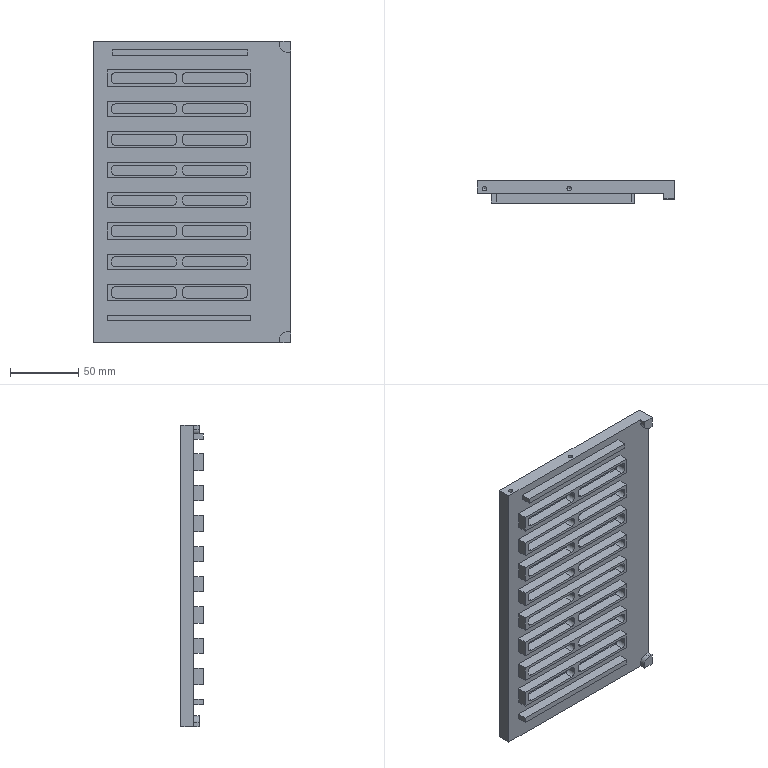NC program | NX | posted with a generic post | part box 144.5 x 16.5 x 221 mm
Whole program:
N10 G17 G21 G94 G90
(DRILLING , TOOL : D8-120)
N12 T19 M6
N14 G54
N16 G17 G0 G90 X-100.5 Y-6. B0. C0. S2000 M3
N18 G43 Z20. H19
N20 G94 G81 G99 Z-0.9 B-180. C-90. F200. R3.
N22 X-32.5
N24 X32.5
N26 X100.5
N28 G80
N30 G0 X100.5 Y-6. Z20.
N32 M5
(DRILLING_COPY , TOOL : 钻头D3.3-45-73)
N34 T09 M6
N36 G54
N38 G17 G0 G90 X-100.5 Y-6. B0. C0. S2000 M3
N40 G43 Z20. H9
N42 G94 G81 G99 Z-9.45 B-180. C-90. F200. R3.
N44 X-32.5
N46 X32.5
N48 X100.5
N50 G80
N52 G0 X100.5 Y-6. Z20.
N54 M5
(DRILLING_COPY_COPY , TOOL : D3.3插刀)
N56 T10 M6
N58 G54
N60 G17 G0 G90 X-100.5 Y-6. B0. C0. S2000 M3
N62 G43 Z20. H10
N64 G94 G81 G99 Z-9.5 B-180. C-90. F200. R3.
N66 X-32.5
N68 X32.5
N70 X100.5
N72 G80
N74 G0 X100.5 Y-6. Z20.
N76 M5
(THREAD_MILLING , TOOL : THREAD_MILL)
N78 T11 M6
N80 G54
N82 G17 G0 G90 X-100.5 Y-6. B0. C0. S3000 M3
N84 G43 Z20. H11
N86 Z-8.675 B-180. C-90.
N88 G41 G94 G3 X-100.35 Y-5.88 Z-8.5 I0.075 J0.06 F200. D11
N90 X-100.35 Y-5.88 Z-7.8 I-0.15 J-0.12
N92 X-100.5 Y-6. Z-7.625 I-0.075 J-0.06
N94 G40
N96 G0 Z-7.275
N98 G41 G3 X-100.35 Y-5.88 Z-7.1 I0.075 J0.06
N100 X-100.35 Y-5.88 Z-6.4 I-0.15 J-0.12
N102 X-100.5 Y-6. Z-6.225 I-0.075 J-0.06
N104 G40
N106 G0 Z-5.875
N108 G41 G3 X-100.35 Y-5.88 Z-5.7 I0.075 J0.06
N110 X-100.35 Y-5.88 Z-5. I-0.15 J-0.12
N112 X-100.5 Y-6. Z-4.825 I-0.075 J-0.06
N114 G40
N116 G0 Z-4.475
N118 G41 G3 X-100.35 Y-5.88 Z-4.3 I0.075 J0.06
N120 X-100.35 Y-5.88 Z-3.6 I-0.15 J-0.12
N122 X-100.5 Y-6. Z-3.425 I-0.075 J-0.06
N124 G40
N126 G0 Z-3.075
N128 G41 G3 X-100.35 Y-5.88 Z-2.9 I0.075 J0.06
N130 X-100.35 Y-5.88 Z-2.2 I-0.15 J-0.12
N132 X-100.5 Y-6. Z-2.025 I-0.075 J-0.06
N134 G40
N136 G0 Z-1.675
N138 G41 G3 X-100.35 Y-5.88 Z-1.5 I0.075 J0.06
N140 X-100.35 Y-5.88 Z-0.8 I-0.15 J-0.12
N142 X-100.35 Y-5.88 Z-0.1 I-0.15 J-0.12
N144 X-100.583 Y-6.173 Z0.3 R-0.192
N146 X-100.5 Y-6. Z0.475 I0.042 J0.086
N148 G40
N150 G0 Z-8.675
N152 G41 G3 X-100.259 Y-5.808 Z-8.5 I0.121 J0.096
N154 X-100.259 Y-5.808 Z-7.8 I-0.241 J-0.192
N156 X-100.5 Y-6. Z-7.625 I-0.121 J-0.096
N158 G40
N160 G0 Z-7.275
N162 G41 G3 X-100.259 Y-5.808 Z-7.1 I0.121 J0.096
N164 X-100.259 Y-5.808 Z-6.4 I-0.241 J-0.192
N166 X-100.5 Y-6. Z-6.225 I-0.121 J-0.096
N168 G40
N170 G0 Z-5.875
N172 G41 G3 X-100.259 Y-5.808 Z-5.7 I0.121 J0.096
N174 X-100.259 Y-5.808 Z-5. I-0.241 J-0.192
N176 X-100.5 Y-6. Z-4.825 I-0.121 J-0.096
N178 G40
N180 G0 Z-4.475
N182 G41 G3 X-100.259 Y-5.808 Z-4.3 I0.121 J0.096
N184 X-100.259 Y-5.808 Z-3.6 I-0.241 J-0.192
N186 X-100.5 Y-6. Z-3.425 I-0.121 J-0.096
N188 G40
N190 G0 Z-3.075
N192 G41 G3 X-100.259 Y-5.808 Z-2.9 I0.121 J0.096
N194 X-100.259 Y-5.808 Z-2.2 I-0.241 J-0.192
N196 X-100.5 Y-6. Z-2.025 I-0.121 J-0.096
N198 G40
N200 G0 Z-1.675
N202 G41 G3 X-100.259 Y-5.808 Z-1.5 I0.121 J0.096
N204 X-100.259 Y-5.808 Z-0.8 I-0.241 J-0.192
N206 X-100.259 Y-5.808 Z-0.1 I-0.241 J-0.192
N208 X-100.634 Y-6.278 Z0.3 R-0.308
N210 X-100.5 Y-6. Z0.475 I0.067 J0.139
N212 G40
N214 G0 Z-8.557
N216 G41 G1 X-100.211 Y-5.921
N218 G3 X-100.168 Y-5.735 Z-8.5 R0.122
N220 X-100.168 Y-5.735 Z-7.8 I-0.332 J-0.265
N222 X-100.358 Y-5.736 Z-7.743 R0.122
N224 G40
N226 G1 X-100.5 Y-6.
N228 G0 Z-7.157
N230 G41 G1 X-100.211 Y-5.921
N232 G3 X-100.168 Y-5.735 Z-7.1 R0.122
N234 X-100.168 Y-5.735 Z-6.4 I-0.332 J-0.265
N236 X-100.358 Y-5.736 Z-6.343 R0.122
N238 G40
N240 G1 X-100.5 Y-6.
N242 G0 Z-5.757
N244 G41 G1 X-100.211 Y-5.921
N246 G3 X-100.168 Y-5.735 Z-5.7 R0.122
N248 X-100.168 Y-5.735 Z-5. I-0.332 J-0.265
N250 X-100.358 Y-5.736 Z-4.943 R0.122
N252 G40
N254 G1 X-100.5 Y-6.
N256 G0 Z-4.357
N258 G41 G1 X-100.211 Y-5.921
N260 G3 X-100.168 Y-5.735 Z-4.3 R0.122
N262 X-100.168 Y-5.735 Z-3.6 I-0.332 J-0.265
N264 X-100.358 Y-5.736 Z-3.543 R0.122
N266 G40
N268 G1 X-100.5 Y-6.
N270 G0 Z-2.957
N272 G41 G1 X-100.211 Y-5.921
N274 G3 X-100.168 Y-5.735 Z-2.9 R0.122
N276 X-100.168 Y-5.735 Z-2.2 I-0.332 J-0.265
N278 X-100.358 Y-5.736 Z-2.143 R0.122
N280 G40
N282 G1 X-100.5 Y-6.
N284 G0 Z-1.557
N286 G41 G1 X-100.211 Y-5.921
N288 G3 X-100.168 Y-5.735 Z-1.5 R0.122
N290 X-100.168 Y-5.735 Z-0.8 I-0.332 J-0.265
N292 X-100.168 Y-5.735 Z-0.1 I-0.332 J-0.265
N294 X-100.684 Y-6.383 Z0.3 R-0.425
N296 X-100.513 Y-6.3 Z0.357 R0.122
N298 G40
N300 G1 X-100.5 Y-6.
N302 G0 Z20.
N304 X-32.5
N306 Z-8.675
N308 G41 G3 X-32.35 Y-5.88 Z-8.5 I0.075 J0.06
N310 X-32.35 Y-5.88 Z-7.8 I-0.15 J-0.12
N312 X-32.5 Y-6. Z-7.625 I-0.075 J-0.06
N314 G40
N316 G0 Z-7.275
N318 G41 G3 X-32.35 Y-5.88 Z-7.1 I0.075 J0.06
N320 X-32.35 Y-5.88 Z-6.4 I-0.15 J-0.12
N322 X-32.5 Y-6. Z-6.225 I-0.075 J-0.06
N324 G40
N326 G0 Z-5.875
N328 G41 G3 X-32.35 Y-5.88 Z-5.7 I0.075 J0.06
N330 X-32.35 Y-5.88 Z-5. I-0.15 J-0.12
N332 X-32.5 Y-6. Z-4.825 I-0.075 J-0.06
N334 G40
N336 G0 Z-4.475
N338 G41 G3 X-32.35 Y-5.88 Z-4.3 I0.075 J0.06
N340 X-32.35 Y-5.88 Z-3.6 I-0.15 J-0.12
N342 X-32.5 Y-6. Z-3.425 I-0.075 J-0.06
N344 G40
N346 G0 Z-3.075
N348 G41 G3 X-32.35 Y-5.88 Z-2.9 I0.075 J0.06
N350 X-32.35 Y-5.88 Z-2.2 I-0.15 J-0.12
N352 X-32.5 Y-6. Z-2.025 I-0.075 J-0.06
N354 G40
N356 G0 Z-1.675
N358 G41 G3 X-32.35 Y-5.88 Z-1.5 I0.075 J0.06
N360 X-32.35 Y-5.88 Z-0.8 I-0.15 J-0.12
N362 X-32.35 Y-5.88 Z-0.1 I-0.15 J-0.12
N364 X-32.583 Y-6.173 Z0.3 R-0.192
N366 X-32.5 Y-6. Z0.475 I0.042 J0.086
N368 G40
N370 G0 Z-8.675
N372 G41 G3 X-32.259 Y-5.808 Z-8.5 I0.121 J0.096
N374 X-32.259 Y-5.808 Z-7.8 I-0.241 J-0.192
N376 X-32.5 Y-6. Z-7.625 I-0.121 J-0.096
N378 G40
N380 G0 Z-7.275
N382 G41 G3 X-32.259 Y-5.808 Z-7.1 I0.121 J0.096
N384 X-32.259 Y-5.808 Z-6.4 I-0.241 J-0.192
N386 X-32.5 Y-6. Z-6.225 I-0.121 J-0.096
N388 G40
N390 G0 Z-5.875
N392 G41 G3 X-32.259 Y-5.808 Z-5.7 I0.121 J0.096
N394 X-32.259 Y-5.808 Z-5. I-0.241 J-0.192
N396 X-32.5 Y-6. Z-4.825 I-0.121 J-0.096
N398 G40
N400 G0 Z-4.475
N402 G41 G3 X-32.259 Y-5.808 Z-4.3 I0.121 J0.096
N404 X-32.259 Y-5.808 Z-3.6 I-0.241 J-0.192
N406 X-32.5 Y-6. Z-3.425 I-0.121 J-0.096
N408 G40
N410 G0 Z-3.075
N412 G41 G3 X-32.259 Y-5.808 Z-2.9 I0.121 J0.096
N414 X-32.259 Y-5.808 Z-2.2 I-0.241 J-0.192
N416 X-32.5 Y-6. Z-2.025 I-0.121 J-0.096
N418 G40
N420 G0 Z-1.675
N422 G41 G3 X-32.259 Y-5.808 Z-1.5 I0.121 J0.096
N424 X-32.259 Y-5.808 Z-0.8 I-0.241 J-0.192
N426 X-32.259 Y-5.808 Z-0.1 I-0.241 J-0.192
N428 X-32.634 Y-6.278 Z0.3 R-0.308
N430 X-32.5 Y-6. Z0.475 I0.067 J0.139
N432 G40
N434 G0 Z-8.557
N436 G41 G1 X-32.211 Y-5.921
N438 G3 X-32.168 Y-5.735 Z-8.5 R0.122
N440 X-32.168 Y-5.735 Z-7.8 I-0.332 J-0.265
N442 X-32.358 Y-5.736 Z-7.743 R0.122
N444 G40
N446 G1 X-32.5 Y-6.
N448 G0 Z-7.157
N450 G41 G1 X-32.211 Y-5.921
N452 G3 X-32.168 Y-5.735 Z-7.1 R0.122
N454 X-32.168 Y-5.735 Z-6.4 I-0.332 J-0.265
N456 X-32.358 Y-5.736 Z-6.343 R0.122
N458 G40
N460 G1 X-32.5 Y-6.
N462 G0 Z-5.757
N464 G41 G1 X-32.211 Y-5.921
N466 G3 X-32.168 Y-5.735 Z-5.7 R0.122
N468 X-32.168 Y-5.735 Z-5. I-0.332 J-0.265
N470 X-32.358 Y-5.736 Z-4.943 R0.122
N472 G40
N474 G1 X-32.5 Y-6.
N476 G0 Z-4.357
N478 G41 G1 X-32.211 Y-5.921
N480 G3 X-32.168 Y-5.735 Z-4.3 R0.122
N482 X-32.168 Y-5.735 Z-3.6 I-0.332 J-0.265
N484 X-32.358 Y-5.736 Z-3.543 R0.122
N486 G40
N488 G1 X-32.5 Y-6.
N490 G0 Z-2.957
N492 G41 G1 X-32.211 Y-5.921
N494 G3 X-32.168 Y-5.735 Z-2.9 R0.122
N496 X-32.168 Y-5.735 Z-2.2 I-0.332 J-0.265
N498 X-32.358 Y-5.736 Z-2.143 R0.122
N500 G40
N502 G1 X-32.5 Y-6.
N504 G0 Z-1.557
N506 G41 G1 X-32.211 Y-5.921
N508 G3 X-32.168 Y-5.735 Z-1.5 R0.122
N510 X-32.168 Y-5.735 Z-0.8 I-0.332 J-0.265
N512 X-32.168 Y-5.735 Z-0.1 I-0.332 J-0.265
N514 X-32.684 Y-6.383 Z0.3 R-0.425
N516 X-32.513 Y-6.3 Z0.357 R0.122
N518 G40
N520 G1 X-32.5 Y-6.
N522 G0 Z20.
N524 X32.5
N526 Z-8.675
N528 G41 G3 X32.65 Y-5.88 Z-8.5 I0.075 J0.06
N530 X32.65 Y-5.88 Z-7.8 I-0.15 J-0.12
N532 X32.5 Y-6. Z-7.625 I-0.075 J-0.06
N534 G40
N536 G0 Z-7.275
N538 G41 G3 X32.65 Y-5.88 Z-7.1 I0.075 J0.06
N540 X32.65 Y-5.88 Z-6.4 I-0.15 J-0.12
N542 X32.5 Y-6. Z-6.225 I-0.075 J-0.06
N544 G40
N546 G0 Z-5.875
N548 G41 G3 X32.65 Y-5.88 Z-5.7 I0.075 J0.06
N550 X32.65 Y-5.88 Z-5. I-0.15 J-0.12
N552 X32.5 Y-6. Z-4.825 I-0.075 J-0.06
N554 G40
N556 G0 Z-4.475
N558 G41 G3 X32.65 Y-5.88 Z-4.3 I0.075 J0.06
N560 X32.65 Y-5.88 Z-3.6 I-0.15 J-0.12
N562 X32.5 Y-6. Z-3.425 I-0.075 J-0.06
N564 G40
N566 G0 Z-3.075
N568 G41 G3 X32.65 Y-5.88 Z-2.9 I0.075 J0.06
N570 X32.65 Y-5.88 Z-2.2 I-0.15 J-0.12
N572 X32.5 Y-6. Z-2.025 I-0.075 J-0.06
N574 G40
N576 G0 Z-1.675
N578 G41 G3 X32.65 Y-5.88 Z-1.5 I0.075 J0.06
N580 X32.65 Y-5.88 Z-0.8 I-0.15 J-0.12
N582 X32.65 Y-5.88 Z-0.1 I-0.15 J-0.12
N584 X32.417 Y-6.173 Z0.3 R-0.192
N586 X32.5 Y-6. Z0.475 I0.042 J0.086
N588 G40
N590 G0 Z-8.675
N592 G41 G3 X32.741 Y-5.808 Z-8.5 I0.121 J0.096
N594 X32.741 Y-5.808 Z-7.8 I-0.241 J-0.192
N596 X32.5 Y-6. Z-7.625 I-0.121 J-0.096
N598 G40
N600 G0 Z-7.275
N602 G41 G3 X32.741 Y-5.808 Z-7.1 I0.121 J0.096
N604 X32.741 Y-5.808 Z-6.4 I-0.241 J-0.192
N606 X32.5 Y-6. Z-6.225 I-0.121 J-0.096
N608 G40
N610 G0 Z-5.875
N612 G41 G3 X32.741 Y-5.808 Z-5.7 I0.121 J0.096
N614 X32.741 Y-5.808 Z-5. I-0.241 J-0.192
N616 X32.5 Y-6. Z-4.825 I-0.121 J-0.096
N618 G40
N620 G0 Z-4.475
N622 G41 G3 X32.741 Y-5.808 Z-4.3 I0.121 J0.096
N624 X32.741 Y-5.808 Z-3.6 I-0.241 J-0.192
N626 X32.5 Y-6. Z-3.425 I-0.121 J-0.096
N628 G40
N630 G0 Z-3.075
N632 G41 G3 X32.741 Y-5.808 Z-2.9 I0.121 J0.096
N634 X32.741 Y-5.808 Z-2.2 I-0.241 J-0.192
N636 X32.5 Y-6. Z-2.025 I-0.121 J-0.096
N638 G40
N640 G0 Z-1.675
N642 G41 G3 X32.741 Y-5.808 Z-1.5 I0.121 J0.096
N644 X32.741 Y-5.808 Z-0.8 I-0.241 J-0.192
N646 X32.741 Y-5.808 Z-0.1 I-0.241 J-0.192
N648 X32.366 Y-6.278 Z0.3 R-0.308
N650 X32.5 Y-6. Z0.475 I0.067 J0.139
N652 G40
N654 G0 Z-8.557
N656 G41 G1 X32.789 Y-5.921
N658 G3 X32.832 Y-5.735 Z-8.5 R0.122
N660 X32.832 Y-5.735 Z-7.8 I-0.332 J-0.265
N662 X32.642 Y-5.736 Z-7.743 R0.122
N664 G40
N666 G1 X32.5 Y-6.
N668 G0 Z-7.157
N670 G41 G1 X32.789 Y-5.921
N672 G3 X32.832 Y-5.735 Z-7.1 R0.122
N674 X32.832 Y-5.735 Z-6.4 I-0.332 J-0.265
N676 X32.642 Y-5.736 Z-6.343 R0.122
N678 G40
N680 G1 X32.5 Y-6.
N682 G0 Z-5.757
N684 G41 G1 X32.789 Y-5.921
N686 G3 X32.832 Y-5.735 Z-5.7 R0.122
N688 X32.832 Y-5.735 Z-5. I-0.332 J-0.265
N690 X32.642 Y-5.736 Z-4.943 R0.122
N692 G40
N694 G1 X32.5 Y-6.
N696 G0 Z-4.357
N698 G41 G1 X32.789 Y-5.921
N700 G3 X32.832 Y-5.735 Z-4.3 R0.122
N702 X32.832 Y-5.735 Z-3.6 I-0.332 J-0.265
N704 X32.642 Y-5.736 Z-3.543 R0.122
N706 G40
N708 G1 X32.5 Y-6.
N710 G0 Z-2.957
N712 G41 G1 X32.789 Y-5.921
N714 G3 X32.832 Y-5.735 Z-2.9 R0.122
N716 X32.832 Y-5.735 Z-2.2 I-0.332 J-0.265
N718 X32.642 Y-5.736 Z-2.143 R0.122
N720 G40
N722 G1 X32.5 Y-6.
N724 G0 Z-1.557
N726 G41 G1 X32.789 Y-5.921
N728 G3 X32.832 Y-5.735 Z-1.5 R0.122
N730 X32.832 Y-5.735 Z-0.8 I-0.332 J-0.265
N732 X32.832 Y-5.735 Z-0.1 I-0.332 J-0.265
N734 X32.316 Y-6.383 Z0.3 R-0.425
N736 X32.487 Y-6.3 Z0.357 R0.122
N738 G40
N740 G1 X32.5 Y-6.
N742 G0 Z20.
N744 X100.5
N746 Z-8.675
N748 G41 G3 X100.65 Y-5.88 Z-8.5 I0.075 J0.06
N750 X100.65 Y-5.88 Z-7.8 I-0.15 J-0.12
N752 X100.5 Y-6. Z-7.625 I-0.075 J-0.06
N754 G40
N756 G0 Z-7.275
N758 G41 G3 X100.65 Y-5.88 Z-7.1 I0.075 J0.06
N760 X100.65 Y-5.88 Z-6.4 I-0.15 J-0.12
N762 X100.5 Y-6. Z-6.225 I-0.075 J-0.06
N764 G40
N766 G0 Z-5.875
N768 G41 G3 X100.65 Y-5.88 Z-5.7 I0.075 J0.06
N770 X100.65 Y-5.88 Z-5. I-0.15 J-0.12
N772 X100.5 Y-6. Z-4.825 I-0.075 J-0.06
N774 G40
N776 G0 Z-4.475
N778 G41 G3 X100.65 Y-5.88 Z-4.3 I0.075 J0.06
N780 X100.65 Y-5.88 Z-3.6 I-0.15 J-0.12
N782 X100.5 Y-6. Z-3.425 I-0.075 J-0.06
N784 G40
N786 G0 Z-3.075
N788 G41 G3 X100.65 Y-5.88 Z-2.9 I0.075 J0.06
N790 X100.65 Y-5.88 Z-2.2 I-0.15 J-0.12
N792 X100.5 Y-6. Z-2.025 I-0.075 J-0.06
N794 G40
N796 G0 Z-1.675
N798 G41 G3 X100.65 Y-5.88 Z-1.5 I0.075 J0.06
N800 X100.65 Y-5.88 Z-0.8 I-0.15 J-0.12
N802 X100.65 Y-5.88 Z-0.1 I-0.15 J-0.12
N804 X100.417 Y-6.173 Z0.3 R-0.192
N806 X100.5 Y-6. Z0.475 I0.042 J0.086
N808 G40
N810 G0 Z-8.675
N812 G41 G3 X100.741 Y-5.808 Z-8.5 I0.121 J0.096
N814 X100.741 Y-5.808 Z-7.8 I-0.241 J-0.192
N816 X100.5 Y-6. Z-7.625 I-0.121 J-0.096
N818 G40
N820 G0 Z-7.275
N822 G41 G3 X100.741 Y-5.808 Z-7.1 I0.121 J0.096
N824 X100.741 Y-5.808 Z-6.4 I-0.241 J-0.192
N826 X100.5 Y-6. Z-6.225 I-0.121 J-0.096
N828 G40
N830 G0 Z-5.875
N832 G41 G3 X100.741 Y-5.808 Z-5.7 I0.121 J0.096
N834 X100.741 Y-5.808 Z-5. I-0.241 J-0.192
N836 X100.5 Y-6. Z-4.825 I-0.121 J-0.096
N838 G40
N840 G0 Z-4.475
N842 G41 G3 X100.741 Y-5.808 Z-4.3 I0.121 J0.096
N844 X100.741 Y-5.808 Z-3.6 I-0.241 J-0.192
N846 X100.5 Y-6. Z-3.425 I-0.121 J-0.096
N848 G40
N850 G0 Z-3.075
N852 G41 G3 X100.741 Y-5.808 Z-2.9 I0.121 J0.096
N854 X100.741 Y-5.808 Z-2.2 I-0.241 J-0.192
N856 X100.5 Y-6. Z-2.025 I-0.121 J-0.096
N858 G40
N860 G0 Z-1.675
N862 G41 G3 X100.741 Y-5.808 Z-1.5 I0.121 J0.096
N864 X100.741 Y-5.808 Z-0.8 I-0.241 J-0.192
N866 X100.741 Y-5.808 Z-0.1 I-0.241 J-0.192
N868 X100.366 Y-6.278 Z0.3 R-0.308
N870 X100.5 Y-6. Z0.475 I0.067 J0.139
N872 G40
N874 G0 Z-8.557
N876 G41 G1 X100.789 Y-5.921
N878 G3 X100.832 Y-5.735 Z-8.5 R0.122
N880 X100.832 Y-5.735 Z-7.8 I-0.332 J-0.265
N882 X100.642 Y-5.736 Z-7.743 R0.122
N884 G40
N886 G1 X100.5 Y-6.
N888 G0 Z-7.157
N890 G41 G1 X100.789 Y-5.921
N892 G3 X100.832 Y-5.735 Z-7.1 R0.122
N894 X100.832 Y-5.735 Z-6.4 I-0.332 J-0.265
N896 X100.642 Y-5.736 Z-6.343 R0.122
N898 G40
N900 G1 X100.5 Y-6.
N902 G0 Z-5.757
N904 G41 G1 X100.789 Y-5.921
N906 G3 X100.832 Y-5.735 Z-5.7 R0.122
N908 X100.832 Y-5.735 Z-5. I-0.332 J-0.265
N910 X100.642 Y-5.736 Z-4.943 R0.122
N912 G40
N914 G1 X100.5 Y-6.
N916 G0 Z-4.357
N918 G41 G1 X100.789 Y-5.921
N920 G3 X100.832 Y-5.735 Z-4.3 R0.122
N922 X100.832 Y-5.735 Z-3.6 I-0.332 J-0.265
N924 X100.642 Y-5.736 Z-3.543 R0.122
N926 G40
N928 G1 X100.5 Y-6.
N930 G0 Z-2.957
N932 G41 G1 X100.789 Y-5.921
N934 G3 X100.832 Y-5.735 Z-2.9 R0.122
N936 X100.832 Y-5.735 Z-2.2 I-0.332 J-0.265
N938 X100.642 Y-5.736 Z-2.143 R0.122
N940 G40
N942 G1 X100.5 Y-6.
N944 G0 Z-1.557
N946 G41 G1 X100.789 Y-5.921
N948 G3 X100.832 Y-5.735 Z-1.5 R0.122
N950 X100.832 Y-5.735 Z-0.8 I-0.332 J-0.265
N952 X100.832 Y-5.735 Z-0.1 I-0.332 J-0.265
N954 X100.316 Y-6.383 Z0.3 R-0.425
N956 X100.487 Y-6.3 Z0.357 R0.122
N958 G40
N960 G1 X100.5 Y-6.
N962 G0 Z20.
N964 M5
(DRILLING_COPY_COPY_COPY , TOOL : 上排M4-13-D5-52)
N966 M6
N968 G54
N970 G17 G0 G90 X-100.5 Y-6. B0. C0. S2000 M3
N972 G43 Z20. H11
N974 G94 G81 G99 Z-9.2 B-180. C-90. F200. R3.
N976 X-32.5
N978 X32.5
N980 X100.5
N982 G80
N984 G0 X100.5 Y-6. Z20.
N986 M5
N988 M2